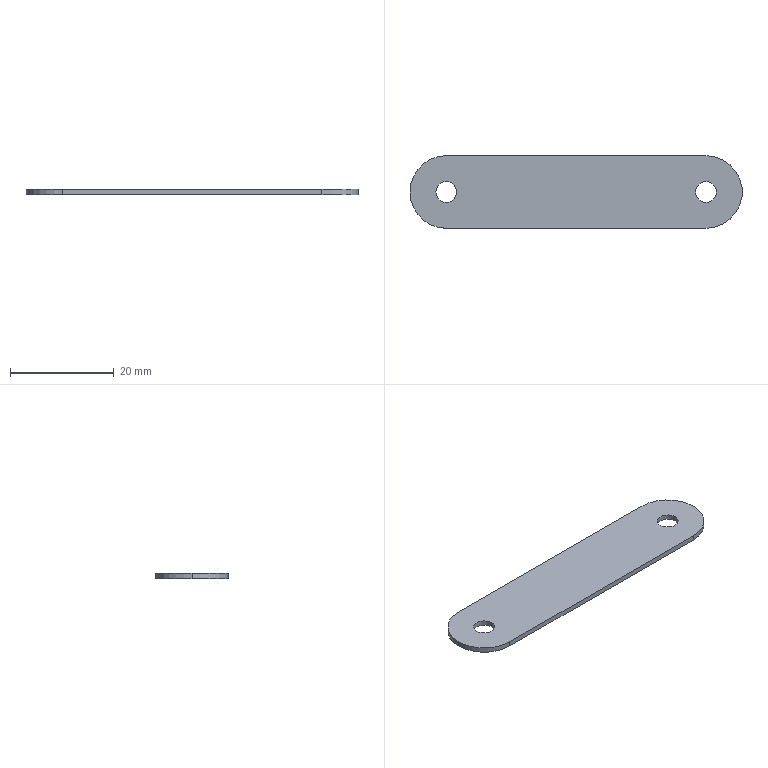Part | SolidWorks | features Extrusion 1 | 1 solid | 11 faces | box 64 x 14 x 1 mm | volume 828.805 mm3 | cylinder 7 | plane 4 | commonest cylinder face diameters 4 x4 14 x3
STEP:
#1=CARTESIAN_POINT('',(14.861,0.,1.));
#2=VERTEX_POINT('',#1);
#3=CARTESIAN_POINT('',(18.861,0.,1.));
#4=VERTEX_POINT('',#3);
#5=CARTESIAN_POINT('',(16.861,0.,1.));
#6=DIRECTION('',(0.,0.,1.));
#7=DIRECTION('',(1.,0.,0.));
#8=AXIS2_PLACEMENT_3D('',#5,#6,#7);
#9=CIRCLE('',#8,2.);
#10=EDGE_CURVE('',#2,#4,#9,.T.);
#11=ORIENTED_EDGE('',*,*,#10,.T.);
#12=CARTESIAN_POINT('',(18.861,0.,0.));
#13=VERTEX_POINT('',#12);
#14=CARTESIAN_POINT('',(18.861,0.,1.));
#15=DIRECTION('',(0.,0.,-1.));
#16=VECTOR('',#15,1000.);
#17=LINE('',#14,#16);
#18=EDGE_CURVE('',#4,#13,#17,.T.);
#19=ORIENTED_EDGE('',*,*,#18,.T.);
#20=CARTESIAN_POINT('',(14.861,0.,0.));
#21=VERTEX_POINT('',#20);
#22=CARTESIAN_POINT('',(16.861,0.,0.));
#23=DIRECTION('',(0.,0.,1.));
#24=DIRECTION('',(1.,0.,0.));
#25=AXIS2_PLACEMENT_3D('',#22,#23,#24);
#26=CIRCLE('',#25,2.);
#27=EDGE_CURVE('',#21,#13,#26,.T.);
#28=ORIENTED_EDGE('',*,*,#27,.F.);
#29=CARTESIAN_POINT('',(14.861,0.,1.));
#30=DIRECTION('',(0.,0.,-1.));
#31=VECTOR('',#30,1000.);
#32=LINE('',#29,#31);
#33=EDGE_CURVE('',#2,#21,#32,.T.);
#34=ORIENTED_EDGE('',*,*,#33,.F.);
#35=EDGE_LOOP('',(#11,#19,#28,#34));
#36=FACE_OUTER_BOUND('',#35,.T.);
#37=CARTESIAN_POINT('',(16.861,0.,1.));
#38=DIRECTION('',(0.,0.,-1.));
#39=DIRECTION('',(-1.,0.,0.));
#40=AXIS2_PLACEMENT_3D('',#37,#38,#39);
#41=CYLINDRICAL_SURFACE('',#40,2.);
#42=ADVANCED_FACE('',(#36),#41,.F.);
#43=CARTESIAN_POINT('',(-35.139,0.,1.));
#44=VERTEX_POINT('',#43);
#45=CARTESIAN_POINT('',(-31.139,0.,1.));
#46=VERTEX_POINT('',#45);
#47=CARTESIAN_POINT('',(-33.139,0.,1.));
#48=DIRECTION('',(0.,0.,1.));
#49=DIRECTION('',(1.,0.,0.));
#50=AXIS2_PLACEMENT_3D('',#47,#48,#49);
#51=CIRCLE('',#50,2.);
#52=EDGE_CURVE('',#44,#46,#51,.T.);
#53=ORIENTED_EDGE('',*,*,#52,.T.);
#54=CARTESIAN_POINT('',(-31.139,0.,0.));
#55=VERTEX_POINT('',#54);
#56=CARTESIAN_POINT('',(-31.139,0.,1.));
#57=DIRECTION('',(0.,0.,-1.));
#58=VECTOR('',#57,1000.);
#59=LINE('',#56,#58);
#60=EDGE_CURVE('',#46,#55,#59,.T.);
#61=ORIENTED_EDGE('',*,*,#60,.T.);
#62=CARTESIAN_POINT('',(-35.139,0.,0.));
#63=VERTEX_POINT('',#62);
#64=CARTESIAN_POINT('',(-33.139,0.,0.));
#65=DIRECTION('',(0.,0.,1.));
#66=DIRECTION('',(1.,0.,0.));
#67=AXIS2_PLACEMENT_3D('',#64,#65,#66);
#68=CIRCLE('',#67,2.);
#69=EDGE_CURVE('',#63,#55,#68,.T.);
#70=ORIENTED_EDGE('',*,*,#69,.F.);
#71=CARTESIAN_POINT('',(-35.139,0.,1.));
#72=DIRECTION('',(0.,0.,-1.));
#73=VECTOR('',#72,1000.);
#74=LINE('',#71,#73);
#75=EDGE_CURVE('',#44,#63,#74,.T.);
#76=ORIENTED_EDGE('',*,*,#75,.F.);
#77=EDGE_LOOP('',(#53,#61,#70,#76));
#78=FACE_OUTER_BOUND('',#77,.T.);
#79=CARTESIAN_POINT('',(-33.139,0.,1.));
#80=DIRECTION('',(0.,0.,-1.));
#81=DIRECTION('',(-1.,0.,0.));
#82=AXIS2_PLACEMENT_3D('',#79,#80,#81);
#83=CYLINDRICAL_SURFACE('',#82,2.);
#84=ADVANCED_FACE('',(#78),#83,.F.);
#85=CARTESIAN_POINT('',(-40.139,0.,1.));
#86=VERTEX_POINT('',#85);
#87=CARTESIAN_POINT('',(-33.139,-7.,1.));
#88=VERTEX_POINT('',#87);
#89=CARTESIAN_POINT('',(-33.139,0.,1.));
#90=DIRECTION('',(0.,0.,1.));
#91=DIRECTION('',(1.,0.,0.));
#92=AXIS2_PLACEMENT_3D('',#89,#90,#91);
#93=CIRCLE('',#92,7.);
#94=EDGE_CURVE('',#86,#88,#93,.T.);
#95=ORIENTED_EDGE('',*,*,#94,.F.);
#96=CARTESIAN_POINT('',(-40.139,0.,0.));
#97=VERTEX_POINT('',#96);
#98=CARTESIAN_POINT('',(-40.139,0.,1.));
#99=DIRECTION('',(0.,0.,-1.));
#100=VECTOR('',#99,1000.);
#101=LINE('',#98,#100);
#102=EDGE_CURVE('',#86,#97,#101,.T.);
#103=ORIENTED_EDGE('',*,*,#102,.T.);
#104=CARTESIAN_POINT('',(-33.139,-7.,0.));
#105=VERTEX_POINT('',#104);
#106=CARTESIAN_POINT('',(-33.139,0.,0.));
#107=DIRECTION('',(0.,0.,1.));
#108=DIRECTION('',(1.,0.,0.));
#109=AXIS2_PLACEMENT_3D('',#106,#107,#108);
#110=CIRCLE('',#109,7.);
#111=EDGE_CURVE('',#97,#105,#110,.T.);
#112=ORIENTED_EDGE('',*,*,#111,.T.);
#113=CARTESIAN_POINT('',(-33.139,-7.,1.));
#114=DIRECTION('',(0.,0.,-1.));
#115=VECTOR('',#114,1000.);
#116=LINE('',#113,#115);
#117=EDGE_CURVE('',#88,#105,#116,.T.);
#118=ORIENTED_EDGE('',*,*,#117,.F.);
#119=EDGE_LOOP('',(#95,#103,#112,#118));
#120=FACE_OUTER_BOUND('',#119,.T.);
#121=CARTESIAN_POINT('',(-33.139,0.,1.));
#122=DIRECTION('',(0.,0.,-1.));
#123=DIRECTION('',(-1.,0.,0.));
#124=AXIS2_PLACEMENT_3D('',#121,#122,#123);
#125=CYLINDRICAL_SURFACE('',#124,7.);
#126=ADVANCED_FACE('',(#120),#125,.T.);
#127=ORIENTED_EDGE('',*,*,#52,.F.);
#128=CARTESIAN_POINT('',(-33.139,0.,1.));
#129=DIRECTION('',(0.,0.,1.));
#130=DIRECTION('',(1.,0.,0.));
#131=AXIS2_PLACEMENT_3D('',#128,#129,#130);
#132=CIRCLE('',#131,2.);
#133=EDGE_CURVE('',#46,#44,#132,.T.);
#134=ORIENTED_EDGE('',*,*,#133,.F.);
#135=EDGE_LOOP('',(#127,#134));
#136=FACE_BOUND('',#135,.T.);
#137=CARTESIAN_POINT('',(-33.139,7.,1.));
#138=VERTEX_POINT('',#137);
#139=CARTESIAN_POINT('',(-33.139,0.,1.));
#140=DIRECTION('',(0.,0.,1.));
#141=DIRECTION('',(1.,0.,0.));
#142=AXIS2_PLACEMENT_3D('',#139,#140,#141);
#143=CIRCLE('',#142,7.);
#144=EDGE_CURVE('',#138,#86,#143,.T.);
#145=ORIENTED_EDGE('',*,*,#144,.T.);
#146=ORIENTED_EDGE('',*,*,#94,.T.);
#147=CARTESIAN_POINT('',(16.861,-7.,1.));
#148=VERTEX_POINT('',#147);
#149=CARTESIAN_POINT('',(-33.139,-7.,1.));
#150=DIRECTION('',(1.,0.,0.));
#151=VECTOR('',#150,1000.);
#152=LINE('',#149,#151);
#153=EDGE_CURVE('',#88,#148,#152,.T.);
#154=ORIENTED_EDGE('',*,*,#153,.T.);
#155=CARTESIAN_POINT('',(16.861,7.,1.));
#156=VERTEX_POINT('',#155);
#157=CARTESIAN_POINT('',(16.861,0.,1.));
#158=DIRECTION('',(0.,0.,1.));
#159=DIRECTION('',(1.,0.,0.));
#160=AXIS2_PLACEMENT_3D('',#157,#158,#159);
#161=CIRCLE('',#160,7.);
#162=EDGE_CURVE('',#148,#156,#161,.T.);
#163=ORIENTED_EDGE('',*,*,#162,.T.);
#164=CARTESIAN_POINT('',(-33.139,7.,1.));
#165=DIRECTION('',(-1.,0.,0.));
#166=VECTOR('',#165,1000.);
#167=LINE('',#164,#166);
#168=EDGE_CURVE('',#156,#138,#167,.T.);
#169=ORIENTED_EDGE('',*,*,#168,.T.);
#170=EDGE_LOOP('',(#145,#146,#154,#163,#169));
#171=FACE_OUTER_BOUND('',#170,.T.);
#172=ORIENTED_EDGE('',*,*,#10,.F.);
#173=CARTESIAN_POINT('',(16.861,0.,1.));
#174=DIRECTION('',(0.,0.,1.));
#175=DIRECTION('',(1.,0.,0.));
#176=AXIS2_PLACEMENT_3D('',#173,#174,#175);
#177=CIRCLE('',#176,2.);
#178=EDGE_CURVE('',#4,#2,#177,.T.);
#179=ORIENTED_EDGE('',*,*,#178,.F.);
#180=EDGE_LOOP('',(#172,#179));
#181=FACE_BOUND('',#180,.T.);
#182=CARTESIAN_POINT('',(-33.139,0.,1.));
#183=DIRECTION('',(0.,0.,1.));
#184=DIRECTION('',(1.,0.,0.));
#185=AXIS2_PLACEMENT_3D('',#182,#183,#184);
#186=PLANE('',#185);
#187=ADVANCED_FACE('',(#136,#171,#181),#186,.T.);
#188=CARTESIAN_POINT('',(-33.139,7.,0.));
#189=VERTEX_POINT('',#188);
#190=CARTESIAN_POINT('',(-33.139,0.,0.));
#191=DIRECTION('',(0.,0.,1.));
#192=DIRECTION('',(1.,0.,0.));
#193=AXIS2_PLACEMENT_3D('',#190,#191,#192);
#194=CIRCLE('',#193,7.);
#195=EDGE_CURVE('',#189,#97,#194,.T.);
#196=ORIENTED_EDGE('',*,*,#195,.F.);
#197=CARTESIAN_POINT('',(16.861,7.,0.));
#198=VERTEX_POINT('',#197);
#199=CARTESIAN_POINT('',(-33.139,7.,0.));
#200=DIRECTION('',(-1.,0.,0.));
#201=VECTOR('',#200,1000.);
#202=LINE('',#199,#201);
#203=EDGE_CURVE('',#198,#189,#202,.T.);
#204=ORIENTED_EDGE('',*,*,#203,.F.);
#205=CARTESIAN_POINT('',(16.861,-7.,0.));
#206=VERTEX_POINT('',#205);
#207=CARTESIAN_POINT('',(16.861,0.,0.));
#208=DIRECTION('',(0.,0.,1.));
#209=DIRECTION('',(1.,0.,0.));
#210=AXIS2_PLACEMENT_3D('',#207,#208,#209);
#211=CIRCLE('',#210,7.);
#212=EDGE_CURVE('',#206,#198,#211,.T.);
#213=ORIENTED_EDGE('',*,*,#212,.F.);
#214=CARTESIAN_POINT('',(-33.139,-7.,0.));
#215=DIRECTION('',(1.,0.,0.));
#216=VECTOR('',#215,1000.);
#217=LINE('',#214,#216);
#218=EDGE_CURVE('',#105,#206,#217,.T.);
#219=ORIENTED_EDGE('',*,*,#218,.F.);
#220=ORIENTED_EDGE('',*,*,#111,.F.);
#221=EDGE_LOOP('',(#196,#204,#213,#219,#220));
#222=FACE_OUTER_BOUND('',#221,.T.);
#223=ORIENTED_EDGE('',*,*,#69,.T.);
#224=CARTESIAN_POINT('',(-33.139,0.,0.));
#225=DIRECTION('',(0.,0.,1.));
#226=DIRECTION('',(1.,0.,0.));
#227=AXIS2_PLACEMENT_3D('',#224,#225,#226);
#228=CIRCLE('',#227,2.);
#229=EDGE_CURVE('',#55,#63,#228,.T.);
#230=ORIENTED_EDGE('',*,*,#229,.T.);
#231=EDGE_LOOP('',(#223,#230));
#232=FACE_BOUND('',#231,.T.);
#233=ORIENTED_EDGE('',*,*,#27,.T.);
#234=CARTESIAN_POINT('',(16.861,0.,0.));
#235=DIRECTION('',(0.,0.,1.));
#236=DIRECTION('',(1.,0.,0.));
#237=AXIS2_PLACEMENT_3D('',#234,#235,#236);
#238=CIRCLE('',#237,2.);
#239=EDGE_CURVE('',#13,#21,#238,.T.);
#240=ORIENTED_EDGE('',*,*,#239,.T.);
#241=EDGE_LOOP('',(#233,#240));
#242=FACE_BOUND('',#241,.T.);
#243=CARTESIAN_POINT('',(-33.139,0.,0.));
#244=DIRECTION('',(0.,0.,1.));
#245=DIRECTION('',(1.,0.,0.));
#246=AXIS2_PLACEMENT_3D('',#243,#244,#245);
#247=PLANE('',#246);
#248=ADVANCED_FACE('',(#222,#232,#242),#247,.F.);
#249=ORIENTED_EDGE('',*,*,#102,.F.);
#250=ORIENTED_EDGE('',*,*,#144,.F.);
#251=CARTESIAN_POINT('',(-33.139,7.,1.));
#252=DIRECTION('',(0.,0.,-1.));
#253=VECTOR('',#252,1000.);
#254=LINE('',#251,#253);
#255=EDGE_CURVE('',#138,#189,#254,.T.);
#256=ORIENTED_EDGE('',*,*,#255,.T.);
#257=ORIENTED_EDGE('',*,*,#195,.T.);
#258=EDGE_LOOP('',(#249,#250,#256,#257));
#259=FACE_OUTER_BOUND('',#258,.T.);
#260=CARTESIAN_POINT('',(-33.139,0.,1.));
#261=DIRECTION('',(0.,0.,-1.));
#262=DIRECTION('',(-1.,0.,0.));
#263=AXIS2_PLACEMENT_3D('',#260,#261,#262);
#264=CYLINDRICAL_SURFACE('',#263,7.);
#265=ADVANCED_FACE('',(#259),#264,.T.);
#266=ORIENTED_EDGE('',*,*,#218,.T.);
#267=CARTESIAN_POINT('',(16.861,-7.,1.));
#268=DIRECTION('',(0.,0.,-1.));
#269=VECTOR('',#268,1000.);
#270=LINE('',#267,#269);
#271=EDGE_CURVE('',#148,#206,#270,.T.);
#272=ORIENTED_EDGE('',*,*,#271,.F.);
#273=ORIENTED_EDGE('',*,*,#153,.F.);
#274=ORIENTED_EDGE('',*,*,#117,.T.);
#275=EDGE_LOOP('',(#266,#272,#273,#274));
#276=FACE_OUTER_BOUND('',#275,.T.);
#277=CARTESIAN_POINT('',(-33.139,-7.,1.));
#278=DIRECTION('',(0.,1.,0.));
#279=DIRECTION('',(0.,0.,1.));
#280=AXIS2_PLACEMENT_3D('',#277,#278,#279);
#281=PLANE('',#280);
#282=ADVANCED_FACE('',(#276),#281,.F.);
#283=ORIENTED_EDGE('',*,*,#212,.T.);
#284=CARTESIAN_POINT('',(16.861,7.,1.));
#285=DIRECTION('',(0.,0.,-1.));
#286=VECTOR('',#285,1000.);
#287=LINE('',#284,#286);
#288=EDGE_CURVE('',#156,#198,#287,.T.);
#289=ORIENTED_EDGE('',*,*,#288,.F.);
#290=ORIENTED_EDGE('',*,*,#162,.F.);
#291=ORIENTED_EDGE('',*,*,#271,.T.);
#292=EDGE_LOOP('',(#283,#289,#290,#291));
#293=FACE_OUTER_BOUND('',#292,.T.);
#294=CARTESIAN_POINT('',(16.861,0.,1.));
#295=DIRECTION('',(0.,0.,-1.));
#296=DIRECTION('',(-1.,0.,0.));
#297=AXIS2_PLACEMENT_3D('',#294,#295,#296);
#298=CYLINDRICAL_SURFACE('',#297,7.);
#299=ADVANCED_FACE('',(#293),#298,.T.);
#300=ORIENTED_EDGE('',*,*,#203,.T.);
#301=ORIENTED_EDGE('',*,*,#255,.F.);
#302=ORIENTED_EDGE('',*,*,#168,.F.);
#303=ORIENTED_EDGE('',*,*,#288,.T.);
#304=EDGE_LOOP('',(#300,#301,#302,#303));
#305=FACE_OUTER_BOUND('',#304,.T.);
#306=CARTESIAN_POINT('',(-33.139,7.,1.));
#307=DIRECTION('',(0.,-1.,0.));
#308=DIRECTION('',(0.,0.,-1.));
#309=AXIS2_PLACEMENT_3D('',#306,#307,#308);
#310=PLANE('',#309);
#311=ADVANCED_FACE('',(#305),#310,.F.);
#312=ORIENTED_EDGE('',*,*,#60,.F.);
#313=ORIENTED_EDGE('',*,*,#133,.T.);
#314=ORIENTED_EDGE('',*,*,#75,.T.);
#315=ORIENTED_EDGE('',*,*,#229,.F.);
#316=EDGE_LOOP('',(#312,#313,#314,#315));
#317=FACE_OUTER_BOUND('',#316,.T.);
#318=CARTESIAN_POINT('',(-33.139,0.,1.));
#319=DIRECTION('',(0.,0.,-1.));
#320=DIRECTION('',(-1.,0.,0.));
#321=AXIS2_PLACEMENT_3D('',#318,#319,#320);
#322=CYLINDRICAL_SURFACE('',#321,2.);
#323=ADVANCED_FACE('',(#317),#322,.F.);
#324=ORIENTED_EDGE('',*,*,#18,.F.);
#325=ORIENTED_EDGE('',*,*,#178,.T.);
#326=ORIENTED_EDGE('',*,*,#33,.T.);
#327=ORIENTED_EDGE('',*,*,#239,.F.);
#328=EDGE_LOOP('',(#324,#325,#326,#327));
#329=FACE_OUTER_BOUND('',#328,.T.);
#330=CARTESIAN_POINT('',(16.861,0.,1.));
#331=DIRECTION('',(0.,0.,-1.));
#332=DIRECTION('',(-1.,0.,0.));
#333=AXIS2_PLACEMENT_3D('',#330,#331,#332);
#334=CYLINDRICAL_SURFACE('',#333,2.);
#335=ADVANCED_FACE('',(#329),#334,.F.);
#336=CLOSED_SHELL('',(#42,#84,#126,#187,#248,#265,#282,#299,#311,#323,#335));
#337=MANIFOLD_SOLID_BREP('',#336);
#338=CARTESIAN_POINT('',(0.,0.,0.));
#339=DIRECTION('',(0.,0.,1.));
#340=DIRECTION('',(1.,0.,0.));
#341=AXIS2_PLACEMENT_3D('',#338,#339,#340);
#342=(LENGTH_UNIT()NAMED_UNIT(*)SI_UNIT(.MILLI.,.METRE.));
#343=UNCERTAINTY_MEASURE_WITH_UNIT(LENGTH_MEASURE(0.00001),#342,'','');
#344=(NAMED_UNIT(*)PLANE_ANGLE_UNIT()SI_UNIT($,.RADIAN.));
#345=(NAMED_UNIT(*)SI_UNIT($,.STERADIAN.)SOLID_ANGLE_UNIT());
#346=(GEOMETRIC_REPRESENTATION_CONTEXT(3)GLOBAL_UNCERTAINTY_ASSIGNED_CONTEXT((#343))GLOBAL_UNIT_ASSIGNED_CONTEXT((#342,#344,#345))REPRESENTATION_CONTEXT('',''));
#347=ADVANCED_BREP_SHAPE_REPRESENTATION('',(#337,#341),#346);